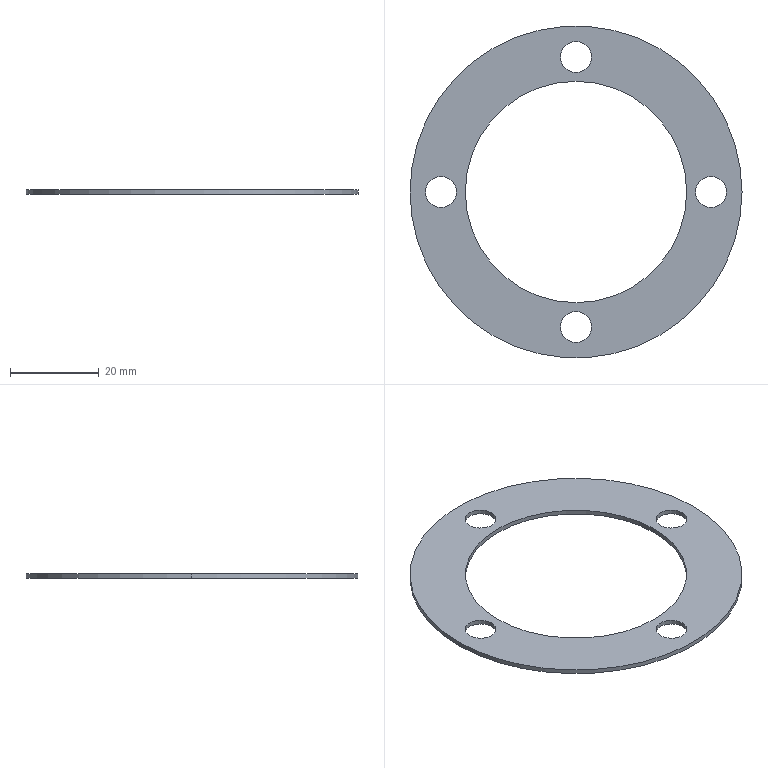Part | SolidWorks | features Extrusion 1 | 1 solid | 14 faces | box 75 x 75 x 1 mm | volume 2300 mm3 | cylinder 12 | plane 2 | commonest cylinder face diameters 7 x8 50 x2 75 x2
STEP:
#1=CARTESIAN_POINT('',(-34.,0.,1.));
#2=VERTEX_POINT('',#1);
#3=CARTESIAN_POINT('',(-27.,0.,1.));
#4=VERTEX_POINT('',#3);
#5=CARTESIAN_POINT('',(-30.5,0.,1.));
#6=DIRECTION('',(0.,0.,1.));
#7=DIRECTION('',(1.,0.,0.));
#8=AXIS2_PLACEMENT_3D('',#5,#6,#7);
#9=CIRCLE('',#8,3.5);
#10=EDGE_CURVE('',#2,#4,#9,.T.);
#11=ORIENTED_EDGE('',*,*,#10,.T.);
#12=CARTESIAN_POINT('',(-27.,0.,0.));
#13=VERTEX_POINT('',#12);
#14=CARTESIAN_POINT('',(-27.,0.,1.));
#15=DIRECTION('',(0.,0.,-1.));
#16=VECTOR('',#15,1000.);
#17=LINE('',#14,#16);
#18=EDGE_CURVE('',#4,#13,#17,.T.);
#19=ORIENTED_EDGE('',*,*,#18,.T.);
#20=CARTESIAN_POINT('',(-34.,0.,0.));
#21=VERTEX_POINT('',#20);
#22=CARTESIAN_POINT('',(-30.5,0.,0.));
#23=DIRECTION('',(0.,0.,1.));
#24=DIRECTION('',(1.,0.,0.));
#25=AXIS2_PLACEMENT_3D('',#22,#23,#24);
#26=CIRCLE('',#25,3.5);
#27=EDGE_CURVE('',#21,#13,#26,.T.);
#28=ORIENTED_EDGE('',*,*,#27,.F.);
#29=CARTESIAN_POINT('',(-34.,0.,1.));
#30=DIRECTION('',(0.,0.,-1.));
#31=VECTOR('',#30,1000.);
#32=LINE('',#29,#31);
#33=EDGE_CURVE('',#2,#21,#32,.T.);
#34=ORIENTED_EDGE('',*,*,#33,.F.);
#35=EDGE_LOOP('',(#11,#19,#28,#34));
#36=FACE_OUTER_BOUND('',#35,.T.);
#37=CARTESIAN_POINT('',(-30.5,0.,1.));
#38=DIRECTION('',(0.,0.,-1.));
#39=DIRECTION('',(-1.,0.,0.));
#40=AXIS2_PLACEMENT_3D('',#37,#38,#39);
#41=CYLINDRICAL_SURFACE('',#40,3.5);
#42=ADVANCED_FACE('',(#36),#41,.F.);
#43=CARTESIAN_POINT('',(-3.5,-30.5,1.));
#44=VERTEX_POINT('',#43);
#45=CARTESIAN_POINT('',(3.5,-30.5,1.));
#46=VERTEX_POINT('',#45);
#47=CARTESIAN_POINT('',(0.,-30.5,1.));
#48=DIRECTION('',(0.,0.,1.));
#49=DIRECTION('',(1.,0.,0.));
#50=AXIS2_PLACEMENT_3D('',#47,#48,#49);
#51=CIRCLE('',#50,3.5);
#52=EDGE_CURVE('',#44,#46,#51,.T.);
#53=ORIENTED_EDGE('',*,*,#52,.T.);
#54=CARTESIAN_POINT('',(3.5,-30.5,0.));
#55=VERTEX_POINT('',#54);
#56=CARTESIAN_POINT('',(3.5,-30.5,1.));
#57=DIRECTION('',(0.,0.,-1.));
#58=VECTOR('',#57,1000.);
#59=LINE('',#56,#58);
#60=EDGE_CURVE('',#46,#55,#59,.T.);
#61=ORIENTED_EDGE('',*,*,#60,.T.);
#62=CARTESIAN_POINT('',(-3.5,-30.5,0.));
#63=VERTEX_POINT('',#62);
#64=CARTESIAN_POINT('',(0.,-30.5,0.));
#65=DIRECTION('',(0.,0.,1.));
#66=DIRECTION('',(1.,0.,0.));
#67=AXIS2_PLACEMENT_3D('',#64,#65,#66);
#68=CIRCLE('',#67,3.5);
#69=EDGE_CURVE('',#63,#55,#68,.T.);
#70=ORIENTED_EDGE('',*,*,#69,.F.);
#71=CARTESIAN_POINT('',(-3.5,-30.5,1.));
#72=DIRECTION('',(0.,0.,-1.));
#73=VECTOR('',#72,1000.);
#74=LINE('',#71,#73);
#75=EDGE_CURVE('',#44,#63,#74,.T.);
#76=ORIENTED_EDGE('',*,*,#75,.F.);
#77=EDGE_LOOP('',(#53,#61,#70,#76));
#78=FACE_OUTER_BOUND('',#77,.T.);
#79=CARTESIAN_POINT('',(0.,-30.5,1.));
#80=DIRECTION('',(0.,0.,-1.));
#81=DIRECTION('',(-1.,0.,0.));
#82=AXIS2_PLACEMENT_3D('',#79,#80,#81);
#83=CYLINDRICAL_SURFACE('',#82,3.5);
#84=ADVANCED_FACE('',(#78),#83,.F.);
#85=CARTESIAN_POINT('',(27.,0.,1.));
#86=VERTEX_POINT('',#85);
#87=CARTESIAN_POINT('',(34.,0.,1.));
#88=VERTEX_POINT('',#87);
#89=CARTESIAN_POINT('',(30.5,0.,1.));
#90=DIRECTION('',(0.,0.,1.));
#91=DIRECTION('',(1.,0.,0.));
#92=AXIS2_PLACEMENT_3D('',#89,#90,#91);
#93=CIRCLE('',#92,3.5);
#94=EDGE_CURVE('',#86,#88,#93,.T.);
#95=ORIENTED_EDGE('',*,*,#94,.T.);
#96=CARTESIAN_POINT('',(34.,0.,0.));
#97=VERTEX_POINT('',#96);
#98=CARTESIAN_POINT('',(34.,0.,1.));
#99=DIRECTION('',(0.,0.,-1.));
#100=VECTOR('',#99,1000.);
#101=LINE('',#98,#100);
#102=EDGE_CURVE('',#88,#97,#101,.T.);
#103=ORIENTED_EDGE('',*,*,#102,.T.);
#104=CARTESIAN_POINT('',(27.,0.,0.));
#105=VERTEX_POINT('',#104);
#106=CARTESIAN_POINT('',(30.5,0.,0.));
#107=DIRECTION('',(0.,0.,1.));
#108=DIRECTION('',(1.,0.,0.));
#109=AXIS2_PLACEMENT_3D('',#106,#107,#108);
#110=CIRCLE('',#109,3.5);
#111=EDGE_CURVE('',#105,#97,#110,.T.);
#112=ORIENTED_EDGE('',*,*,#111,.F.);
#113=CARTESIAN_POINT('',(27.,0.,1.));
#114=DIRECTION('',(0.,0.,-1.));
#115=VECTOR('',#114,1000.);
#116=LINE('',#113,#115);
#117=EDGE_CURVE('',#86,#105,#116,.T.);
#118=ORIENTED_EDGE('',*,*,#117,.F.);
#119=EDGE_LOOP('',(#95,#103,#112,#118));
#120=FACE_OUTER_BOUND('',#119,.T.);
#121=CARTESIAN_POINT('',(30.5,0.,1.));
#122=DIRECTION('',(0.,0.,-1.));
#123=DIRECTION('',(-1.,0.,0.));
#124=AXIS2_PLACEMENT_3D('',#121,#122,#123);
#125=CYLINDRICAL_SURFACE('',#124,3.5);
#126=ADVANCED_FACE('',(#120),#125,.F.);
#127=CARTESIAN_POINT('',(-3.5,30.5,1.));
#128=VERTEX_POINT('',#127);
#129=CARTESIAN_POINT('',(3.5,30.5,1.));
#130=VERTEX_POINT('',#129);
#131=CARTESIAN_POINT('',(0.,30.5,1.));
#132=DIRECTION('',(0.,0.,1.));
#133=DIRECTION('',(1.,0.,0.));
#134=AXIS2_PLACEMENT_3D('',#131,#132,#133);
#135=CIRCLE('',#134,3.5);
#136=EDGE_CURVE('',#128,#130,#135,.T.);
#137=ORIENTED_EDGE('',*,*,#136,.T.);
#138=CARTESIAN_POINT('',(3.5,30.5,0.));
#139=VERTEX_POINT('',#138);
#140=CARTESIAN_POINT('',(3.5,30.5,1.));
#141=DIRECTION('',(0.,0.,-1.));
#142=VECTOR('',#141,1000.);
#143=LINE('',#140,#142);
#144=EDGE_CURVE('',#130,#139,#143,.T.);
#145=ORIENTED_EDGE('',*,*,#144,.T.);
#146=CARTESIAN_POINT('',(-3.5,30.5,0.));
#147=VERTEX_POINT('',#146);
#148=CARTESIAN_POINT('',(0.,30.5,0.));
#149=DIRECTION('',(0.,0.,1.));
#150=DIRECTION('',(1.,0.,0.));
#151=AXIS2_PLACEMENT_3D('',#148,#149,#150);
#152=CIRCLE('',#151,3.5);
#153=EDGE_CURVE('',#147,#139,#152,.T.);
#154=ORIENTED_EDGE('',*,*,#153,.F.);
#155=CARTESIAN_POINT('',(-3.5,30.5,1.));
#156=DIRECTION('',(0.,0.,-1.));
#157=VECTOR('',#156,1000.);
#158=LINE('',#155,#157);
#159=EDGE_CURVE('',#128,#147,#158,.T.);
#160=ORIENTED_EDGE('',*,*,#159,.F.);
#161=EDGE_LOOP('',(#137,#145,#154,#160));
#162=FACE_OUTER_BOUND('',#161,.T.);
#163=CARTESIAN_POINT('',(0.,30.5,1.));
#164=DIRECTION('',(0.,0.,-1.));
#165=DIRECTION('',(-1.,0.,0.));
#166=AXIS2_PLACEMENT_3D('',#163,#164,#165);
#167=CYLINDRICAL_SURFACE('',#166,3.5);
#168=ADVANCED_FACE('',(#162),#167,.F.);
#169=CARTESIAN_POINT('',(-25.,0.,1.));
#170=VERTEX_POINT('',#169);
#171=CARTESIAN_POINT('',(25.,0.,1.));
#172=VERTEX_POINT('',#171);
#173=CARTESIAN_POINT('',(0.,0.,1.));
#174=DIRECTION('',(0.,0.,1.));
#175=DIRECTION('',(1.,0.,0.));
#176=AXIS2_PLACEMENT_3D('',#173,#174,#175);
#177=CIRCLE('',#176,25.);
#178=EDGE_CURVE('',#170,#172,#177,.T.);
#179=ORIENTED_EDGE('',*,*,#178,.T.);
#180=CARTESIAN_POINT('',(25.,0.,0.));
#181=VERTEX_POINT('',#180);
#182=CARTESIAN_POINT('',(25.,0.,1.));
#183=DIRECTION('',(0.,0.,-1.));
#184=VECTOR('',#183,1000.);
#185=LINE('',#182,#184);
#186=EDGE_CURVE('',#172,#181,#185,.T.);
#187=ORIENTED_EDGE('',*,*,#186,.T.);
#188=CARTESIAN_POINT('',(-25.,0.,0.));
#189=VERTEX_POINT('',#188);
#190=CARTESIAN_POINT('',(0.,0.,0.));
#191=DIRECTION('',(0.,0.,1.));
#192=DIRECTION('',(1.,0.,0.));
#193=AXIS2_PLACEMENT_3D('',#190,#191,#192);
#194=CIRCLE('',#193,25.);
#195=EDGE_CURVE('',#189,#181,#194,.T.);
#196=ORIENTED_EDGE('',*,*,#195,.F.);
#197=CARTESIAN_POINT('',(-25.,0.,1.));
#198=DIRECTION('',(0.,0.,-1.));
#199=VECTOR('',#198,1000.);
#200=LINE('',#197,#199);
#201=EDGE_CURVE('',#170,#189,#200,.T.);
#202=ORIENTED_EDGE('',*,*,#201,.F.);
#203=EDGE_LOOP('',(#179,#187,#196,#202));
#204=FACE_OUTER_BOUND('',#203,.T.);
#205=CARTESIAN_POINT('',(0.,0.,1.));
#206=DIRECTION('',(0.,0.,-1.));
#207=DIRECTION('',(-1.,0.,0.));
#208=AXIS2_PLACEMENT_3D('',#205,#206,#207);
#209=CYLINDRICAL_SURFACE('',#208,25.);
#210=ADVANCED_FACE('',(#204),#209,.F.);
#211=CARTESIAN_POINT('',(37.5,0.,1.));
#212=VERTEX_POINT('',#211);
#213=CARTESIAN_POINT('',(-37.5,0.,1.));
#214=VERTEX_POINT('',#213);
#215=CARTESIAN_POINT('',(0.,0.,1.));
#216=DIRECTION('',(0.,0.,1.));
#217=DIRECTION('',(1.,0.,0.));
#218=AXIS2_PLACEMENT_3D('',#215,#216,#217);
#219=CIRCLE('',#218,37.5);
#220=EDGE_CURVE('',#212,#214,#219,.T.);
#221=ORIENTED_EDGE('',*,*,#220,.F.);
#222=CARTESIAN_POINT('',(37.5,0.,0.));
#223=VERTEX_POINT('',#222);
#224=CARTESIAN_POINT('',(37.5,0.,1.));
#225=DIRECTION('',(0.,0.,-1.));
#226=VECTOR('',#225,1000.);
#227=LINE('',#224,#226);
#228=EDGE_CURVE('',#212,#223,#227,.T.);
#229=ORIENTED_EDGE('',*,*,#228,.T.);
#230=CARTESIAN_POINT('',(-37.5,0.,0.));
#231=VERTEX_POINT('',#230);
#232=CARTESIAN_POINT('',(0.,0.,0.));
#233=DIRECTION('',(0.,0.,1.));
#234=DIRECTION('',(1.,0.,0.));
#235=AXIS2_PLACEMENT_3D('',#232,#233,#234);
#236=CIRCLE('',#235,37.5);
#237=EDGE_CURVE('',#223,#231,#236,.T.);
#238=ORIENTED_EDGE('',*,*,#237,.T.);
#239=CARTESIAN_POINT('',(-37.5,0.,1.));
#240=DIRECTION('',(0.,0.,-1.));
#241=VECTOR('',#240,1000.);
#242=LINE('',#239,#241);
#243=EDGE_CURVE('',#214,#231,#242,.T.);
#244=ORIENTED_EDGE('',*,*,#243,.F.);
#245=EDGE_LOOP('',(#221,#229,#238,#244));
#246=FACE_OUTER_BOUND('',#245,.T.);
#247=CARTESIAN_POINT('',(0.,0.,1.));
#248=DIRECTION('',(0.,0.,-1.));
#249=DIRECTION('',(-1.,0.,0.));
#250=AXIS2_PLACEMENT_3D('',#247,#248,#249);
#251=CYLINDRICAL_SURFACE('',#250,37.5);
#252=ADVANCED_FACE('',(#246),#251,.T.);
#253=ORIENTED_EDGE('',*,*,#52,.F.);
#254=CARTESIAN_POINT('',(0.,-30.5,1.));
#255=DIRECTION('',(0.,0.,1.));
#256=DIRECTION('',(1.,0.,0.));
#257=AXIS2_PLACEMENT_3D('',#254,#255,#256);
#258=CIRCLE('',#257,3.5);
#259=EDGE_CURVE('',#46,#44,#258,.T.);
#260=ORIENTED_EDGE('',*,*,#259,.F.);
#261=EDGE_LOOP('',(#253,#260));
#262=FACE_BOUND('',#261,.T.);
#263=ORIENTED_EDGE('',*,*,#136,.F.);
#264=CARTESIAN_POINT('',(0.,30.5,1.));
#265=DIRECTION('',(0.,0.,1.));
#266=DIRECTION('',(1.,0.,0.));
#267=AXIS2_PLACEMENT_3D('',#264,#265,#266);
#268=CIRCLE('',#267,3.5);
#269=EDGE_CURVE('',#130,#128,#268,.T.);
#270=ORIENTED_EDGE('',*,*,#269,.F.);
#271=EDGE_LOOP('',(#263,#270));
#272=FACE_BOUND('',#271,.T.);
#273=CARTESIAN_POINT('',(0.,0.,1.));
#274=DIRECTION('',(0.,0.,1.));
#275=DIRECTION('',(1.,0.,0.));
#276=AXIS2_PLACEMENT_3D('',#273,#274,#275);
#277=CIRCLE('',#276,37.5);
#278=EDGE_CURVE('',#214,#212,#277,.T.);
#279=ORIENTED_EDGE('',*,*,#278,.T.);
#280=ORIENTED_EDGE('',*,*,#220,.T.);
#281=EDGE_LOOP('',(#279,#280));
#282=FACE_OUTER_BOUND('',#281,.T.);
#283=ORIENTED_EDGE('',*,*,#178,.F.);
#284=CARTESIAN_POINT('',(0.,0.,1.));
#285=DIRECTION('',(0.,0.,1.));
#286=DIRECTION('',(1.,0.,0.));
#287=AXIS2_PLACEMENT_3D('',#284,#285,#286);
#288=CIRCLE('',#287,25.);
#289=EDGE_CURVE('',#172,#170,#288,.T.);
#290=ORIENTED_EDGE('',*,*,#289,.F.);
#291=EDGE_LOOP('',(#283,#290));
#292=FACE_BOUND('',#291,.T.);
#293=ORIENTED_EDGE('',*,*,#94,.F.);
#294=CARTESIAN_POINT('',(30.5,0.,1.));
#295=DIRECTION('',(0.,0.,1.));
#296=DIRECTION('',(1.,0.,0.));
#297=AXIS2_PLACEMENT_3D('',#294,#295,#296);
#298=CIRCLE('',#297,3.5);
#299=EDGE_CURVE('',#88,#86,#298,.T.);
#300=ORIENTED_EDGE('',*,*,#299,.F.);
#301=EDGE_LOOP('',(#293,#300));
#302=FACE_BOUND('',#301,.T.);
#303=ORIENTED_EDGE('',*,*,#10,.F.);
#304=CARTESIAN_POINT('',(-30.5,0.,1.));
#305=DIRECTION('',(0.,0.,1.));
#306=DIRECTION('',(1.,0.,0.));
#307=AXIS2_PLACEMENT_3D('',#304,#305,#306);
#308=CIRCLE('',#307,3.5);
#309=EDGE_CURVE('',#4,#2,#308,.T.);
#310=ORIENTED_EDGE('',*,*,#309,.F.);
#311=EDGE_LOOP('',(#303,#310));
#312=FACE_BOUND('',#311,.T.);
#313=CARTESIAN_POINT('',(0.,0.,1.));
#314=DIRECTION('',(0.,0.,1.));
#315=DIRECTION('',(1.,0.,0.));
#316=AXIS2_PLACEMENT_3D('',#313,#314,#315);
#317=PLANE('',#316);
#318=ADVANCED_FACE('',(#262,#272,#282,#292,#302,#312),#317,.T.);
#319=CARTESIAN_POINT('',(0.,0.,0.));
#320=DIRECTION('',(0.,0.,1.));
#321=DIRECTION('',(1.,0.,0.));
#322=AXIS2_PLACEMENT_3D('',#319,#320,#321);
#323=CIRCLE('',#322,37.5);
#324=EDGE_CURVE('',#231,#223,#323,.T.);
#325=ORIENTED_EDGE('',*,*,#324,.F.);
#326=ORIENTED_EDGE('',*,*,#237,.F.);
#327=EDGE_LOOP('',(#325,#326));
#328=FACE_OUTER_BOUND('',#327,.T.);
#329=ORIENTED_EDGE('',*,*,#195,.T.);
#330=CARTESIAN_POINT('',(0.,0.,0.));
#331=DIRECTION('',(0.,0.,1.));
#332=DIRECTION('',(1.,0.,0.));
#333=AXIS2_PLACEMENT_3D('',#330,#331,#332);
#334=CIRCLE('',#333,25.);
#335=EDGE_CURVE('',#181,#189,#334,.T.);
#336=ORIENTED_EDGE('',*,*,#335,.T.);
#337=EDGE_LOOP('',(#329,#336));
#338=FACE_BOUND('',#337,.T.);
#339=ORIENTED_EDGE('',*,*,#153,.T.);
#340=CARTESIAN_POINT('',(0.,30.5,0.));
#341=DIRECTION('',(0.,0.,1.));
#342=DIRECTION('',(1.,0.,0.));
#343=AXIS2_PLACEMENT_3D('',#340,#341,#342);
#344=CIRCLE('',#343,3.5);
#345=EDGE_CURVE('',#139,#147,#344,.T.);
#346=ORIENTED_EDGE('',*,*,#345,.T.);
#347=EDGE_LOOP('',(#339,#346));
#348=FACE_BOUND('',#347,.T.);
#349=ORIENTED_EDGE('',*,*,#111,.T.);
#350=CARTESIAN_POINT('',(30.5,0.,0.));
#351=DIRECTION('',(0.,0.,1.));
#352=DIRECTION('',(1.,0.,0.));
#353=AXIS2_PLACEMENT_3D('',#350,#351,#352);
#354=CIRCLE('',#353,3.5);
#355=EDGE_CURVE('',#97,#105,#354,.T.);
#356=ORIENTED_EDGE('',*,*,#355,.T.);
#357=EDGE_LOOP('',(#349,#356));
#358=FACE_BOUND('',#357,.T.);
#359=ORIENTED_EDGE('',*,*,#69,.T.);
#360=CARTESIAN_POINT('',(0.,-30.5,0.));
#361=DIRECTION('',(0.,0.,1.));
#362=DIRECTION('',(1.,0.,0.));
#363=AXIS2_PLACEMENT_3D('',#360,#361,#362);
#364=CIRCLE('',#363,3.5);
#365=EDGE_CURVE('',#55,#63,#364,.T.);
#366=ORIENTED_EDGE('',*,*,#365,.T.);
#367=EDGE_LOOP('',(#359,#366));
#368=FACE_BOUND('',#367,.T.);
#369=ORIENTED_EDGE('',*,*,#27,.T.);
#370=CARTESIAN_POINT('',(-30.5,0.,0.));
#371=DIRECTION('',(0.,0.,1.));
#372=DIRECTION('',(1.,0.,0.));
#373=AXIS2_PLACEMENT_3D('',#370,#371,#372);
#374=CIRCLE('',#373,3.5);
#375=EDGE_CURVE('',#13,#21,#374,.T.);
#376=ORIENTED_EDGE('',*,*,#375,.T.);
#377=EDGE_LOOP('',(#369,#376));
#378=FACE_BOUND('',#377,.T.);
#379=CARTESIAN_POINT('',(0.,0.,0.));
#380=DIRECTION('',(0.,0.,1.));
#381=DIRECTION('',(1.,0.,0.));
#382=AXIS2_PLACEMENT_3D('',#379,#380,#381);
#383=PLANE('',#382);
#384=ADVANCED_FACE('',(#328,#338,#348,#358,#368,#378),#383,.F.);
#385=ORIENTED_EDGE('',*,*,#228,.F.);
#386=ORIENTED_EDGE('',*,*,#278,.F.);
#387=ORIENTED_EDGE('',*,*,#243,.T.);
#388=ORIENTED_EDGE('',*,*,#324,.T.);
#389=EDGE_LOOP('',(#385,#386,#387,#388));
#390=FACE_OUTER_BOUND('',#389,.T.);
#391=CARTESIAN_POINT('',(0.,0.,1.));
#392=DIRECTION('',(0.,0.,-1.));
#393=DIRECTION('',(-1.,0.,0.));
#394=AXIS2_PLACEMENT_3D('',#391,#392,#393);
#395=CYLINDRICAL_SURFACE('',#394,37.5);
#396=ADVANCED_FACE('',(#390),#395,.T.);
#397=ORIENTED_EDGE('',*,*,#186,.F.);
#398=ORIENTED_EDGE('',*,*,#289,.T.);
#399=ORIENTED_EDGE('',*,*,#201,.T.);
#400=ORIENTED_EDGE('',*,*,#335,.F.);
#401=EDGE_LOOP('',(#397,#398,#399,#400));
#402=FACE_OUTER_BOUND('',#401,.T.);
#403=CARTESIAN_POINT('',(0.,0.,1.));
#404=DIRECTION('',(0.,0.,-1.));
#405=DIRECTION('',(-1.,0.,0.));
#406=AXIS2_PLACEMENT_3D('',#403,#404,#405);
#407=CYLINDRICAL_SURFACE('',#406,25.);
#408=ADVANCED_FACE('',(#402),#407,.F.);
#409=ORIENTED_EDGE('',*,*,#144,.F.);
#410=ORIENTED_EDGE('',*,*,#269,.T.);
#411=ORIENTED_EDGE('',*,*,#159,.T.);
#412=ORIENTED_EDGE('',*,*,#345,.F.);
#413=EDGE_LOOP('',(#409,#410,#411,#412));
#414=FACE_OUTER_BOUND('',#413,.T.);
#415=CARTESIAN_POINT('',(0.,30.5,1.));
#416=DIRECTION('',(0.,0.,-1.));
#417=DIRECTION('',(-1.,0.,0.));
#418=AXIS2_PLACEMENT_3D('',#415,#416,#417);
#419=CYLINDRICAL_SURFACE('',#418,3.5);
#420=ADVANCED_FACE('',(#414),#419,.F.);
#421=ORIENTED_EDGE('',*,*,#102,.F.);
#422=ORIENTED_EDGE('',*,*,#299,.T.);
#423=ORIENTED_EDGE('',*,*,#117,.T.);
#424=ORIENTED_EDGE('',*,*,#355,.F.);
#425=EDGE_LOOP('',(#421,#422,#423,#424));
#426=FACE_OUTER_BOUND('',#425,.T.);
#427=CARTESIAN_POINT('',(30.5,0.,1.));
#428=DIRECTION('',(0.,0.,-1.));
#429=DIRECTION('',(-1.,0.,0.));
#430=AXIS2_PLACEMENT_3D('',#427,#428,#429);
#431=CYLINDRICAL_SURFACE('',#430,3.5);
#432=ADVANCED_FACE('',(#426),#431,.F.);
#433=ORIENTED_EDGE('',*,*,#60,.F.);
#434=ORIENTED_EDGE('',*,*,#259,.T.);
#435=ORIENTED_EDGE('',*,*,#75,.T.);
#436=ORIENTED_EDGE('',*,*,#365,.F.);
#437=EDGE_LOOP('',(#433,#434,#435,#436));
#438=FACE_OUTER_BOUND('',#437,.T.);
#439=CARTESIAN_POINT('',(0.,-30.5,1.));
#440=DIRECTION('',(0.,0.,-1.));
#441=DIRECTION('',(-1.,0.,0.));
#442=AXIS2_PLACEMENT_3D('',#439,#440,#441);
#443=CYLINDRICAL_SURFACE('',#442,3.5);
#444=ADVANCED_FACE('',(#438),#443,.F.);
#445=ORIENTED_EDGE('',*,*,#18,.F.);
#446=ORIENTED_EDGE('',*,*,#309,.T.);
#447=ORIENTED_EDGE('',*,*,#33,.T.);
#448=ORIENTED_EDGE('',*,*,#375,.F.);
#449=EDGE_LOOP('',(#445,#446,#447,#448));
#450=FACE_OUTER_BOUND('',#449,.T.);
#451=CARTESIAN_POINT('',(-30.5,0.,1.));
#452=DIRECTION('',(0.,0.,-1.));
#453=DIRECTION('',(-1.,0.,0.));
#454=AXIS2_PLACEMENT_3D('',#451,#452,#453);
#455=CYLINDRICAL_SURFACE('',#454,3.5);
#456=ADVANCED_FACE('',(#450),#455,.F.);
#457=CLOSED_SHELL('',(#42,#84,#126,#168,#210,#252,#318,#384,#396,#408,#420,#432,#444,#456));
#458=MANIFOLD_SOLID_BREP('',#457);
#459=CARTESIAN_POINT('',(0.,0.,0.));
#460=DIRECTION('',(0.,0.,1.));
#461=DIRECTION('',(1.,0.,0.));
#462=AXIS2_PLACEMENT_3D('',#459,#460,#461);
#463=(LENGTH_UNIT()NAMED_UNIT(*)SI_UNIT(.MILLI.,.METRE.));
#464=UNCERTAINTY_MEASURE_WITH_UNIT(LENGTH_MEASURE(0.00001),#463,'','');
#465=(NAMED_UNIT(*)PLANE_ANGLE_UNIT()SI_UNIT($,.RADIAN.));
#466=(NAMED_UNIT(*)SI_UNIT($,.STERADIAN.)SOLID_ANGLE_UNIT());
#467=(GEOMETRIC_REPRESENTATION_CONTEXT(3)GLOBAL_UNCERTAINTY_ASSIGNED_CONTEXT((#464))GLOBAL_UNIT_ASSIGNED_CONTEXT((#463,#465,#466))REPRESENTATION_CONTEXT('',''));
#468=ADVANCED_BREP_SHAPE_REPRESENTATION('',(#458,#462),#467);